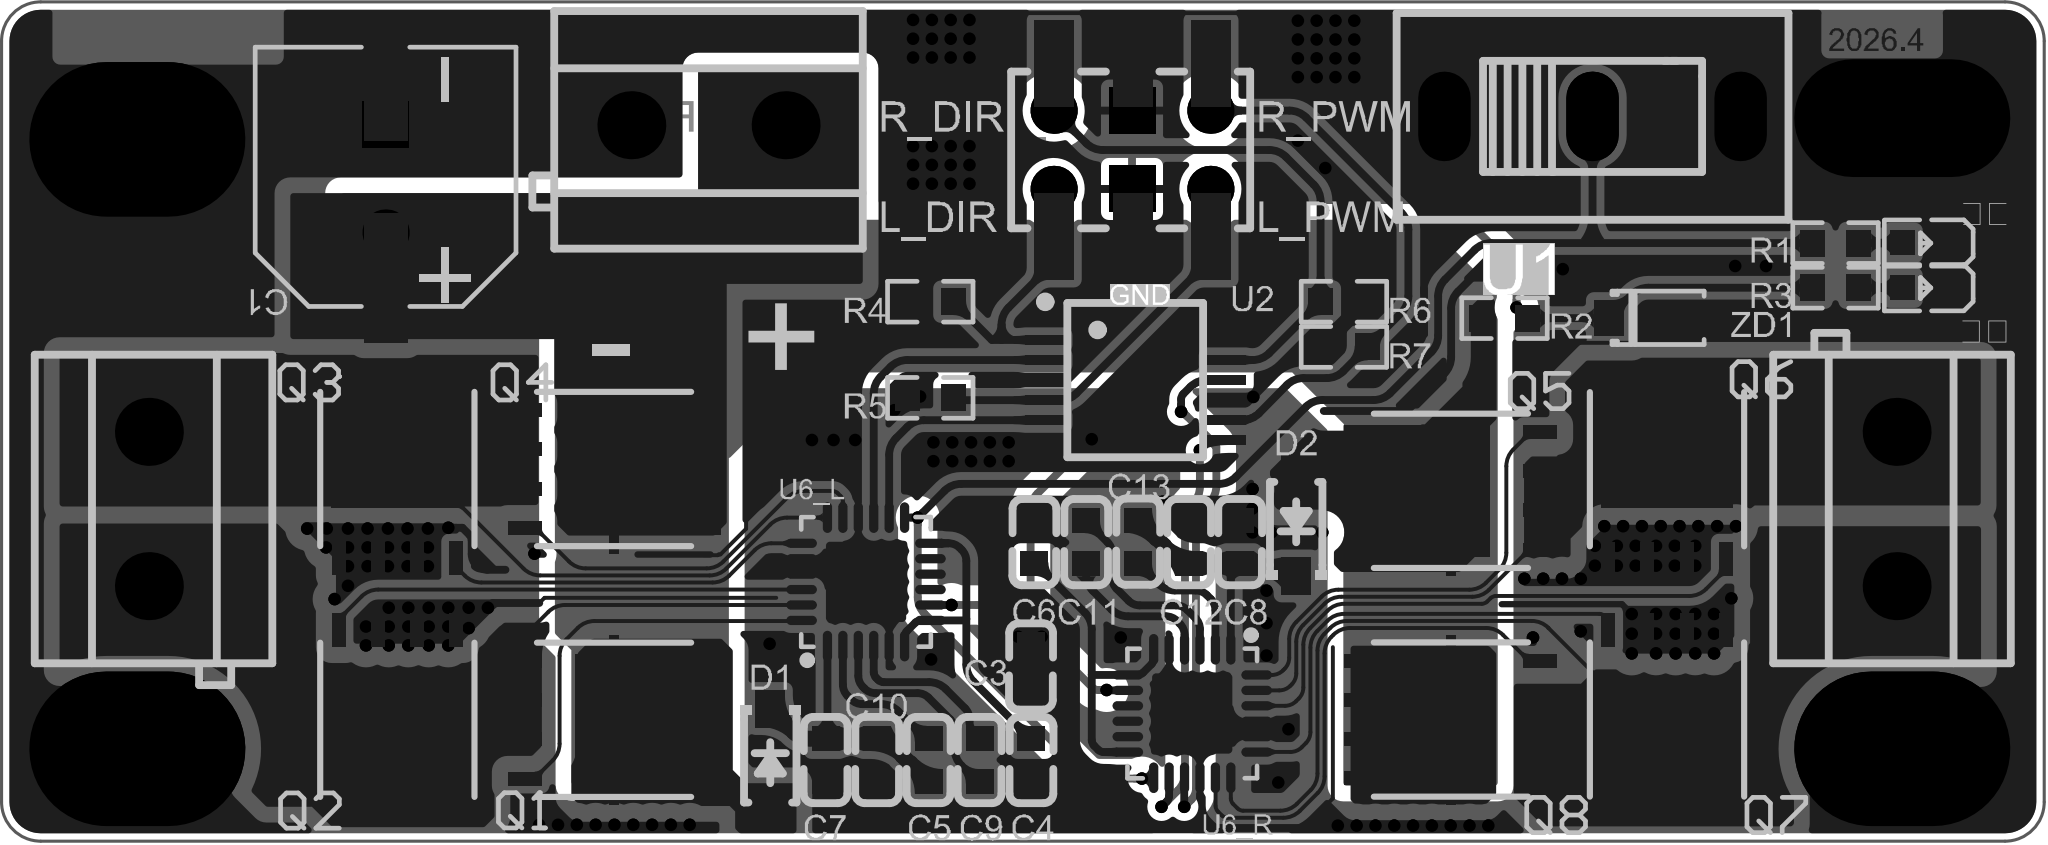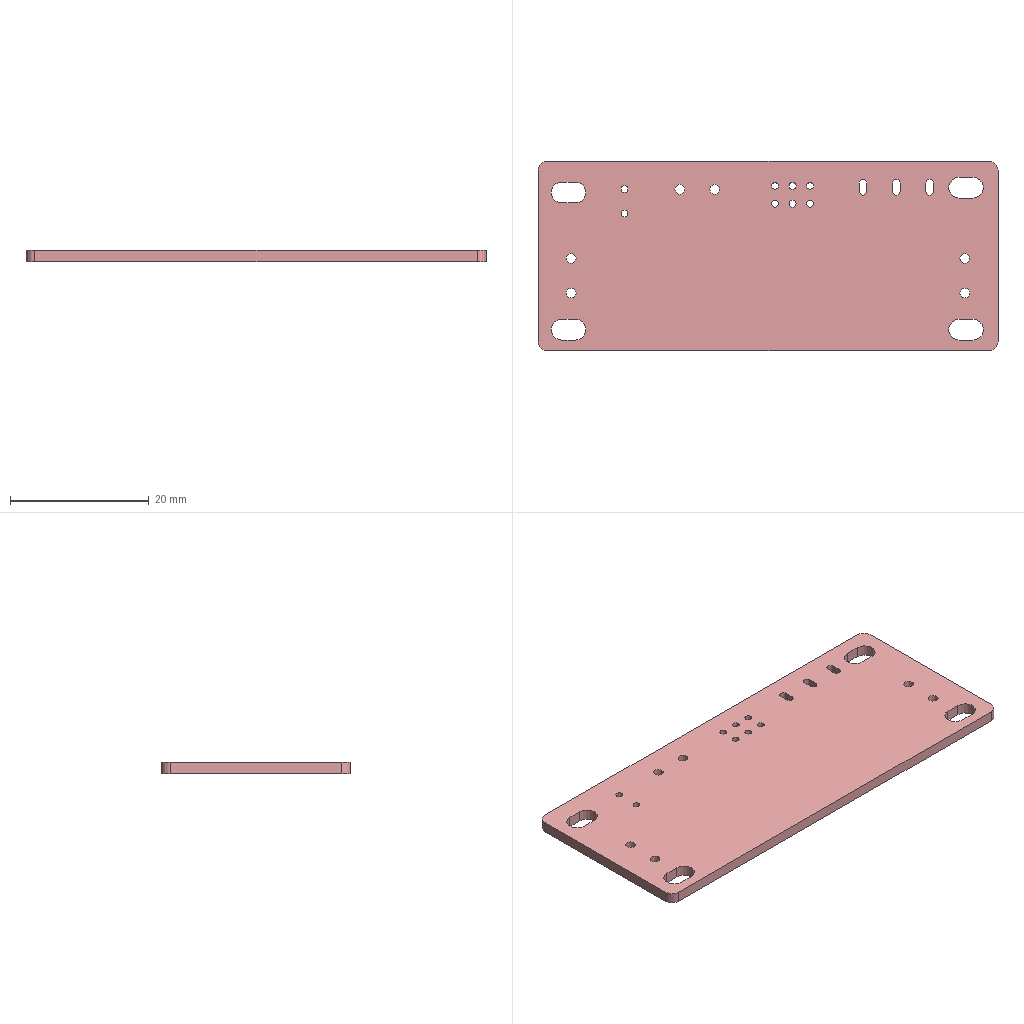Circuit board layout | Altium Designer | box 66.2 x 27.2 x 1.6 mm
Layer stack:
# Altium Designer layer stack of  (unit mm; dielectric type: 0 none, 1 core, 2 prepreg, 3 surface material)
index,name,kind,layer,copper_thickness_mm,dielectric_type,dielectric_thickness_mm,dielectric_material,dielectric_constant
0,Top Paste Mask Layer,other,,,,,,
1,Top Silkscreen Layer,other,,,,,,
2,Top Solder Mask Layer,dielectric,,,3,0.01,,3.3
3,Top Layer,copper,Top Layer,0.035,,,,
4,Dielectric1,dielectric,,,3,1.51,FR4,4.5
5,Bottom Layer,copper,Bottom Layer,0.035,,,,
6,Bottom Solder Mask Layer,dielectric,,,3,0.01,,3.3
7,Bottom Silkscreen Layer,other,,,,,,
8,Bottom Paste Mask Layer,other,,,,,,
# drill layer pairs: low layer,high layer
drill_pair,Top Layer,Bottom Layer
Part placement:
Designator,Comment,Layer,Footprint,Center-X(mm),Center-Y(mm),Rotation
C1,220uF,TopLayer,CAP-SMD_BD8.0-L8.3-W8.3-FD,88.646,97.826,90
C2,220uF,TopLayer,CAP-TH_BD8.0-P3.50-D0.6-FD,88.646,97.769,90
C3,1UF,TopLayer,C0603,109.566,81.964,90
C4,1UF,TopLayer,C0603,109.576,78.916,270
C5,1UF,TopLayer,C0603,106.248,78.932,90
C6,1UF,TopLayer,C0603,109.674,85.994,90
C7,10UF,TopLayer,C0603,102.904,78.916,270
C8,10UF,TopLayer,C0603,116.341,85.994,90
C9,100nF,TopLayer,C0603,107.902,78.932,90
C10,100nF,TopLayer,C0603,104.576,78.916,270
C11,100nF,TopLayer,C0603,111.348,85.979,270
C12,100nF,TopLayer,C0603,114.687,85.994,90
C13,1UF,TopLayer,C0603,113.033,85.994,270
D1,1N5819W,TopLayer,SOD-123_L2.7-W1.6-LS3.7-RD-1,101.112,78.894,270
D2,1N5819W,TopLayer,SOD-123_L2.7-W1.6-LS3.7-RD-1,118.158,86.59,90
H1,贴片,TopLayer,HDR-SMD_6P-P2.54-V-M-R2-C5-S7.4,112.856,98.696,0
K1,KF301-5.0-2P,TopLayer,CONN-TH_P5.00_KF301-5.0-2P,99.111,99.498,180
K2,KF301-5.0-2P,TopLayer,CONN-TH_P5.00_KF301-5.0-2P,137.617,87.06,90
K3,KF301-5.0-2P,TopLayer,CONN-TH_P5.00_KF301-5.0-2P,80.975,87.06,270
??,,TopLayer,LED_0603,138.608,94.236,180
M1,,TopLayer,M4螺丝,80.6,99.038,0
M2,,TopLayer,M4螺丝,137.8,99.727,0
M3,,TopLayer,M4螺丝,80.6,79.288,0
M4,,TopLayer,M4螺丝,137.8,79.288,0
R1,2.2K,TopLayer,R0603,135.636,95.679,180
R2,2.2K,TopLayer,R0603,124.908,93.246,180
R3,2.2K,TopLayer,R0603,135.636,94.231,180
R4,10K,TopLayer,R0603,106.299,93.778,180
R5,10K,TopLayer,R0603,106.299,90.662,180
R6,10K,TopLayer,R0603,119.705,93.778,180
R7,10K,TopLayer,R0603,119.705,92.313,0
U1,SS12D10G5,TopLayer,SW-TH_SHOU-HAN_SS12D10G4,127.762,99.783,0
U2,SN74HC125PWR,TopLayer,TSSOP-14_L5.0-W4.4-P0.65-LS6.5-BL,112.953,91.237,270
U6_L,DRV8701ERGET,TopLayer,VQFN-24_L4.0-W4.0-P0.50-BL-EP2.5,104.216,84.699,0
U6_R,DRV8701ERGET,TopLayer,VQFN-24_L4.0-W4.0-P0.50-BL-EP2.5,114.789,80.432,180
ZD1,BZT52C3V6,TopLayer,SOD-123_L2.8-W1.8-LS3.7-RD,129.972,93.256,0
??,,TopLayer,LED_0603,138.608,95.684,180
H2,,TopLayer,HDR-TH_6P-P2.54-V-R2-C3-S2.54_A2541WV-2X3P,112.837,98.701,0
Q1,TPH1R403NL,TopLayer,DFN5x6,95.925,80.228,270
Q2,TPH1R403NL,TopLayer,DFN5x6,89.027,80.353,180
Q3,TPH1R403NL,TopLayer,DFN5x6,89.027,88.231,0
Q4,TPH1R403NL,TopLayer,DFN5x6,95.925,88.356,270
Q5,TPH1R403NL,TopLayer,DFN5x6,123.297,87.649,90
Q6,TPH1R403NL,TopLayer,DFN5x6,130.175,88.224,0
Q7,TPH1R403NL,TopLayer,DFN5x6,130.175,80.363,180
Q8,TPH1R403NL,TopLayer,DFN5x6,123.297,80.238,90
Pad and via stacks:
# Altium Designer via and pad stacks of  (unit mm). Each distinct definition once, with the count of objects using it.
# via: kind,start_layer,end_layer,hole_mm,diameter_mm,mode(0 simple;1 top-mid-bottom;2 full stack),diameter_per_layer,count,example_net
# pad: kind,layer,hole_mm,hole_type(0 round;1 square;2 slot),plating,top_size,top_shape(1 round;2 rect;3 octagon;9 rounded rect),mid_size,bottom_size,mode,footprint,size_per_layer,count,example
pad,Top Layer,0,0,plated,4.2x1.4,2,4.2x1.4,4.2x1.4,0,CAP-SMD_BD8.0-L8.3-W8.3-FD,,2,C1.1
pad,Top Layer,0,0,plated,0.8x0.9,2,0.8x0.9,0.8x0.9,0,C0603,,22,C3.2
pad,Top Layer,0,0,plated,1.2x0.95,2,1.2x0.95,1.2x0.95,0,SOD-123_L2.7-W1.6-LS3.7-RD-1,,4,D1.2
pad,Top Layer,0,0,plated,1.27x2.8,2,1.27x2.8,1.27x2.8,0,HDR-SMD_6P-P2.54-V-M-R2-C5-S7.4,,6,H1.1
pad,Top Layer,0,0,plated,0.8001x0.8001,2,0.8001x0.8001,0.8001x0.8001,0,LED_0603,,4,\u7535\u6E90.1
pad,Top Layer,0,0,plated,0.8065x0.864,2,0.8065x0.864,0.8065x0.864,0,R0603,,14,R1.2
pad,Top Layer,0,0,plated,0.3048x1.27,2,0.3048x1.27,0.3048x1.27,0,TSSOP-14_L5.0-W4.4-P0.65-LS6.5-BL,,14,U2.1
pad,Top Layer,0,0,plated,2.6x2.6,9,2.6x2.6,2.6x2.6,0,VQFN-24_L4.0-W4.0-P0.50-BL-EP2.5,,2,U6_L.25
pad,Top Layer,0,0,plated,0.3x0.9906,9,0.3x0.9906,0.3x0.9906,0,VQFN-24_L4.0-W4.0-P0.50-BL-EP2.5,,48,U6_L.24
pad,Top Layer,0,0,plated,0.95x1.15,2,0.95x1.15,0.95x1.15,0,SOD-123_L2.8-W1.8-LS3.7-RD,,2,ZD1.2
pad,Top Layer,0,0,plated,4.25x3.5,2,4.25x3.5,4.25x3.5,0,DFN5x6,,8,Q1.1
pad,Top Layer,0,0,plated,0.45x1.6,2,0.45x1.6,0.45x1.6,0,DFN5x6,,32,Q1.1
pad,Top Layer,0,0,plated,0.45x1.1,2,0.45x1.1,0.45x1.1,0,DFN5x6,,32,Q1.3
pad,Top Layer,0,0,plated,5.5x0.3,2,5.5x0.3,5.5x0.3,0,DFN5x6,,8,Q1.1
pad,Multi-Layer,0.9906,0,plated,1.499x1.499,2,1.499x1.499,1.499x1.499,0,CAP-TH_BD8.0-P3.50-D0.6-FD,,1,C2.2
pad,Multi-Layer,0.9906,0,plated,1.499x1.499,1,1.499x1.499,1.499x1.499,0,CAP-TH_BD8.0-P3.50-D0.6-FD,,1,C2.1
pad,Multi-Layer,1.4,0,plated,2.2x2.2,1,2.2x2.2,2.2x2.2,0,CONN-TH_P5.00_KF301-5.0-2P,,6,K1.1
pad,Multi-Layer,3,2,plated,7x5,1,7x5,7x5,0,M4\u00C2\u00DD\u00CB\u00BF,,3,M1.1
pad,Multi-Layer,3,2,plated,7x3.81,1,7x3.81,7x3.81,0,M4\u00C2\u00DD\u00CB\u00BF,,1,M2.1
pad,Multi-Layer,1.1,2,plated,1.7x2.9,1,1.7x2.9,1.7x2.9,0,SW-TH_SHOU-HAN_SS12D10G4,,3,U1.1
pad,Multi-Layer,0.9906,0,plated,1.499x1.499,1,1.499x1.499,1.499x1.499,0,HDR-TH_6P-P2.54-V-R2-C3-S2.54_A2541WV-2X3P,,4,H2.1
pad,Multi-Layer,0.9906,0,plated,1.499x1.499,2,1.499x1.499,1.499x1.499,0,HDR-TH_6P-P2.54-V-R2-C3-S2.54_A2541WV-2X3P,,2,H2.3
via,Top Layer,Bottom Layer,0.3048,0.4064,0,,514,GND
Copper pours:
name,layer,net,type(0 solid;1 hatched;2 none)
Top Layer-VM,Top Layer,VM,0
Top Layer-VM 1,Top Layer,VM,0
Top Layer-L_A,Top Layer,L_A,0
Top Layer-R_A,Top Layer,R_A,0
Top Layer-R_B,Top Layer,R_B,0
Top Layer-VM 2,Top Layer,VM,0
Top Layer-VM 3,Top Layer,VM,0
Top Layer-VM 4,Top Layer,VM,0
Top Layer-GND,Top Layer,GND,0
Top Layer-L_B,Top Layer,L_B,0
Bottom Layer-VM,Bottom Layer,VM,0
Bottom Layer-VM 1,Bottom Layer,VM,0
Bottom Layer-VM 2,Bottom Layer,VM,0
Bottom Layer-VM 3,Bottom Layer,VM,0
Bottom Layer-GND,Bottom Layer,GND,0
Bottom Layer-R_A,Bottom Layer,R_A,0
Bottom Layer-R_B,Bottom Layer,R_B,0
Bottom Layer-L_B,Bottom Layer,L_B,0
Bottom Layer-L_A,Bottom Layer,L_A,0
Design rules, without the lines most boards share:
# Altium Designer design rules of  (exported by Altium Designer, unit mm)
# columns: name | kind | enabled | priority | scope1 | scope2 | descriptor | typed fields (field=value)
copperThickness2oz | 0 | disabled | 1 | All | All | Clearance Constraint (Gap=6mil) (Disabled)(All),(All) | gap=0.1524
Plane_innerPlane | 0 | disabled | 2 | All | All | Clearance Constraint (Gap=6mil) (Disabled)(All),(All) | gap=0.1524
Copper_copperRegion | 0 | disabled | 3 | All | All | Clearance Constraint (Gap=6mil) (Disabled)(All),(All) | gap=0.1524
Clearance | 0 | disabled | 4 | All | All | Clearance Constraint (Gap=6mil) (Disabled)(All),(All) | gap=0.1524
BoardOutlineClearance | 63 | disabled | 4 | All | All | Board Clearance Constraint (Gap=0mil) (Disabled)(All) |
Copper_18 | 0 | disabled | 5 | All | All | Clearance Constraint (Gap=6mil) (Disabled)(All),(All) | gap=0.1524
Copper_18_1 | 63 | disabled | 5 | All | All | Board Clearance Constraint (Gap=0mil) (Disabled)(All) |
copperThickness1oz | 0 | enabled | 6 | All | All | Clearance Constraint (Gap=6mil) (All),(All) | gap=0.1524
copperThickness1oz_1 | 63 | enabled | 6 | All | All | Board Clearance Constraint (Gap=0mil) (All) |
otherClearance | 52 | enabled | 1 | All | All | Hole To Hole Clearance (Gap=11.8mil) (All),(All) | gap=0.2997
viaSize | 11 | enabled | 1 | All | All | Routing Via (MinHoleWidth=11.8mil) (MaxHoleWidth=248mil) (PreferredHoleWidth=12mil) (MinWidth=15.7mil) (MaxWidth=393.7mil) (PreferedWidth=24mil) (All) | via_min_hole=0.2997 via_max_hole=6.299 via_preferred_diameter=0.6096 via_preferred_hole=0.3048
PolygonConnect | 20 | disabled | 1 | All | All | Polygon Connect Rule(Direct Connect )(Conductor Width=10mil) (Relief Angle=90 Angle) (Entries=4) (Air Gap Width=10mil) (Disabled)(All),(All) | connect_style(0=relief,1=direct,2=none)=1 relief_conductor_width=0.254 relief_entries=4
18 | 20 | disabled | 2 | All | All | Polygon Connect Rule(Relief Connect )(Conductor Width=10mil) (Relief Angle=90 Angle) (Entries=4) (Air Gap Width=10mil) (Disabled)(All),(All) | connect_style(0=relief,1=direct,2=none)=0 relief_conductor_width=0.254 relief_entries=4
copperRegion | 20 | enabled | 3 | All | All | Polygon Connect Rule(Relief Connect )(Conductor Width=10mil) (Relief Angle=90 Angle) (Entries=4) (Air Gap Width=10mil) (All),(All) | connect_style(0=relief,1=direct,2=none)=0 relief_conductor_width=0.254 relief_entries=4